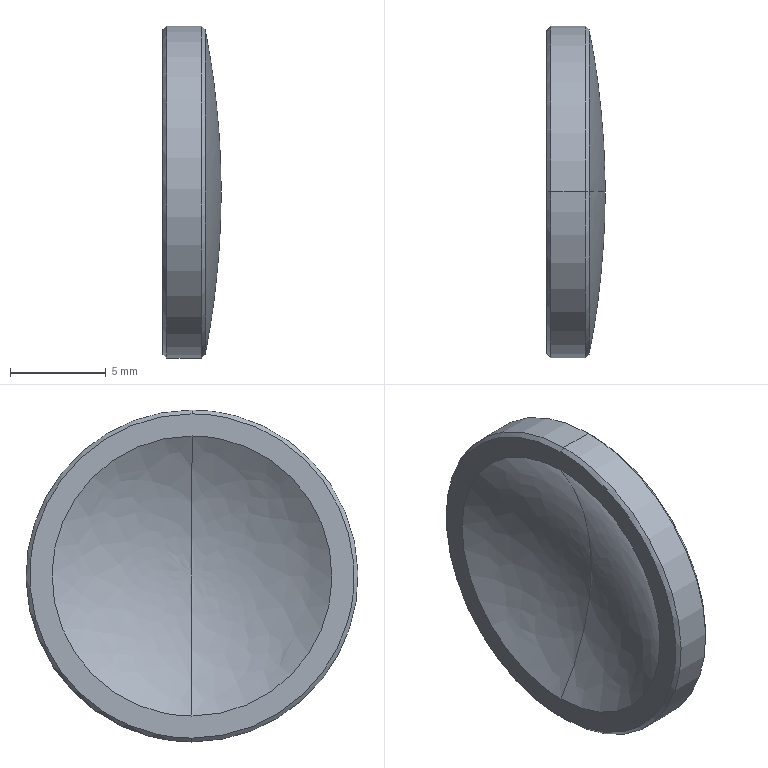Part | SolidWorks | features BaseBody 1 | 1 solid | 11 faces | box 3.031 x 17.3 x 17.3 mm | volume 416.795 mm3 | spline 11
STEP:
#1=CARTESIAN_POINT('',(5.315,0.,-8.45));
#2=VERTEX_POINT('',#1);
#3=CARTESIAN_POINT('',(6.141,0.,0.));
#4=VERTEX_POINT('',#3);
#5=CARTESIAN_POINT('',(-37.512,0.,0.));
#6=DIRECTION('',(0.,-1.,0.));
#7=DIRECTION('',(0.9803,0.,-0.1974));
#8=AXIS2_PLACEMENT_3D('',#5,#6,#7);
#9=CIRCLE('',#8,43.653);
#10=EDGE_CURVE('',#2,#4,#9,.T.);
#11=ORIENTED_EDGE('',*,*,#10,.F.);
#12=CARTESIAN_POINT('',(5.315,0.,8.45));
#13=VERTEX_POINT('',#12);
#14=CARTESIAN_POINT('',(5.315,0.,8.45));
#15=CARTESIAN_POINT('',(5.315,16.9,8.45));
#16=CARTESIAN_POINT('',(5.315,16.9,-8.45));
#17=CARTESIAN_POINT('',(5.315,0.,-8.45));
#18=(BOUNDED_CURVE()B_SPLINE_CURVE(3,(#14,#15,#16,#17),.UNSPECIFIED.,.F.,.F.)B_SPLINE_CURVE_WITH_KNOTS((4,4),(0.,51.9),.UNSPECIFIED.)CURVE()GEOMETRIC_REPRESENTATION_ITEM()RATIONAL_B_SPLINE_CURVE((1.,0.3333,0.3333,1.))REPRESENTATION_ITEM(''));
#19=EDGE_CURVE('',#13,#2,#18,.T.);
#20=ORIENTED_EDGE('',*,*,#19,.F.);
#21=CARTESIAN_POINT('',(-37.512,0.,0.));
#22=DIRECTION('',(0.,1.,0.));
#23=DIRECTION('',(0.9803,0.,0.1974));
#24=AXIS2_PLACEMENT_3D('',#21,#22,#23);
#25=CIRCLE('',#24,43.653);
#26=EDGE_CURVE('',#13,#4,#25,.T.);
#27=ORIENTED_EDGE('',*,*,#26,.T.);
#28=EDGE_LOOP('',(#11,#20,#27));
#29=FACE_OUTER_BOUND('',#28,.T.);
#30=CARTESIAN_POINT('',(5.315,0.,-8.45));
#31=CARTESIAN_POINT('',(5.315,16.9,-8.45));
#32=CARTESIAN_POINT('',(5.315,16.9,8.45));
#33=CARTESIAN_POINT('',(5.315,0.,8.45));
#34=CARTESIAN_POINT('',(5.865,0.,-5.665));
#35=CARTESIAN_POINT('',(5.865,11.329,-5.665));
#36=CARTESIAN_POINT('',(5.865,11.329,5.665));
#37=CARTESIAN_POINT('',(5.865,0.,5.665));
#38=CARTESIAN_POINT('',(6.141,0.,-2.839));
#39=CARTESIAN_POINT('',(6.141,5.678,-2.839));
#40=CARTESIAN_POINT('',(6.141,5.678,2.839));
#41=CARTESIAN_POINT('',(6.141,0.,2.839));
#42=CARTESIAN_POINT('',(6.141,0.,0.));
#43=CARTESIAN_POINT('',(6.141,0.,0.));
#44=CARTESIAN_POINT('',(6.141,0.,0.));
#45=CARTESIAN_POINT('',(6.141,0.,0.));
#46=(BOUNDED_SURFACE()B_SPLINE_SURFACE(3,3,((#30,#31,#32,#33),(#34,#35,#36,#37),(#38,#39,#40,#41),(#42,#43,#44,#45)),.UNSPECIFIED.,.F.,.F.,.T.)B_SPLINE_SURFACE_WITH_KNOTS((4,4),(4,4),(0.,1.),(0.,1.),.UNSPECIFIED.)GEOMETRIC_REPRESENTATION_ITEM()RATIONAL_B_SPLINE_SURFACE(((1.,0.3333,0.3333,1.),(0.9968,0.3323,0.3323,0.9968),(0.9968,0.3323,0.3323,0.9968),(1.,0.3333,0.3333,1.)))REPRESENTATION_ITEM('')SURFACE());
#47=ADVANCED_FACE('',(#29),#46,.F.);
#48=ORIENTED_EDGE('',*,*,#26,.F.);
#49=CARTESIAN_POINT('',(5.315,0.,-8.45));
#50=CARTESIAN_POINT('',(5.315,-16.9,-8.45));
#51=CARTESIAN_POINT('',(5.315,-16.9,8.45));
#52=CARTESIAN_POINT('',(5.315,0.,8.45));
#53=(BOUNDED_CURVE()B_SPLINE_CURVE(3,(#49,#50,#51,#52),.UNSPECIFIED.,.F.,.F.)B_SPLINE_CURVE_WITH_KNOTS((4,4),(0.,51.9),.UNSPECIFIED.)CURVE()GEOMETRIC_REPRESENTATION_ITEM()RATIONAL_B_SPLINE_CURVE((1.,0.3333,0.3333,1.))REPRESENTATION_ITEM(''));
#54=EDGE_CURVE('',#2,#13,#53,.T.);
#55=ORIENTED_EDGE('',*,*,#54,.F.);
#56=ORIENTED_EDGE('',*,*,#10,.T.);
#57=EDGE_LOOP('',(#48,#55,#56));
#58=FACE_OUTER_BOUND('',#57,.T.);
#59=CARTESIAN_POINT('',(5.315,0.,8.45));
#60=CARTESIAN_POINT('',(5.315,-16.9,8.45));
#61=CARTESIAN_POINT('',(5.315,-16.9,-8.45));
#62=CARTESIAN_POINT('',(5.315,0.,-8.45));
#63=CARTESIAN_POINT('',(5.865,0.,5.665));
#64=CARTESIAN_POINT('',(5.865,-11.329,5.665));
#65=CARTESIAN_POINT('',(5.865,-11.329,-5.665));
#66=CARTESIAN_POINT('',(5.865,0.,-5.665));
#67=CARTESIAN_POINT('',(6.141,0.,2.839));
#68=CARTESIAN_POINT('',(6.141,-5.678,2.839));
#69=CARTESIAN_POINT('',(6.141,-5.678,-2.839));
#70=CARTESIAN_POINT('',(6.141,0.,-2.839));
#71=CARTESIAN_POINT('',(6.141,0.,0.));
#72=CARTESIAN_POINT('',(6.141,0.,0.));
#73=CARTESIAN_POINT('',(6.141,0.,0.));
#74=CARTESIAN_POINT('',(6.141,0.,0.));
#75=(BOUNDED_SURFACE()B_SPLINE_SURFACE(3,3,((#59,#60,#61,#62),(#63,#64,#65,#66),(#67,#68,#69,#70),(#71,#72,#73,#74)),.UNSPECIFIED.,.F.,.F.,.F.)B_SPLINE_SURFACE_WITH_KNOTS((4,4),(4,4),(0.,1.),(0.,1.),.UNSPECIFIED.)GEOMETRIC_REPRESENTATION_ITEM()RATIONAL_B_SPLINE_SURFACE(((1.,0.3333,0.3333,1.),(0.9968,0.3323,0.3323,0.9968),(0.9968,0.3323,0.3323,0.9968),(1.,0.3333,0.3333,1.)))REPRESENTATION_ITEM('')SURFACE());
#76=ADVANCED_FACE('',(#58),#75,.F.);
#77=CARTESIAN_POINT('',(5.115,0.,-8.65));
#78=VERTEX_POINT('',#77);
#79=CARTESIAN_POINT('',(5.315,0.,-8.45));
#80=DIRECTION('',(-0.7071,0.,-0.7071));
#81=VECTOR('',#80,1000.);
#82=LINE('',#79,#81);
#83=EDGE_CURVE('',#2,#78,#82,.T.);
#84=ORIENTED_EDGE('',*,*,#83,.F.);
#85=ORIENTED_EDGE('',*,*,#54,.T.);
#86=CARTESIAN_POINT('',(5.115,0.,8.65));
#87=VERTEX_POINT('',#86);
#88=CARTESIAN_POINT('',(5.315,0.,8.45));
#89=DIRECTION('',(-0.7071,0.,0.7071));
#90=VECTOR('',#89,1000.);
#91=LINE('',#88,#90);
#92=EDGE_CURVE('',#13,#87,#91,.T.);
#93=ORIENTED_EDGE('',*,*,#92,.T.);
#94=CARTESIAN_POINT('',(5.115,0.,-8.65));
#95=CARTESIAN_POINT('',(5.115,-17.3,-8.65));
#96=CARTESIAN_POINT('',(5.115,-17.3,8.65));
#97=CARTESIAN_POINT('',(5.115,0.,8.65));
#98=(BOUNDED_CURVE()B_SPLINE_CURVE(3,(#94,#95,#96,#97),.UNSPECIFIED.,.F.,.F.)B_SPLINE_CURVE_WITH_KNOTS((4,4),(0.,51.9),.UNSPECIFIED.)CURVE()GEOMETRIC_REPRESENTATION_ITEM()RATIONAL_B_SPLINE_CURVE((1.,0.3333,0.3333,1.))REPRESENTATION_ITEM(''));
#99=EDGE_CURVE('',#78,#87,#98,.T.);
#100=ORIENTED_EDGE('',*,*,#99,.F.);
#101=EDGE_LOOP('',(#84,#85,#93,#100));
#102=FACE_OUTER_BOUND('',#101,.T.);
#103=CARTESIAN_POINT('',(5.315,0.,-8.45));
#104=CARTESIAN_POINT('',(5.315,-16.9,-8.45));
#105=CARTESIAN_POINT('',(5.315,-16.9,8.45));
#106=CARTESIAN_POINT('',(5.315,0.,8.45));
#107=CARTESIAN_POINT('',(5.115,0.,-8.65));
#108=CARTESIAN_POINT('',(5.115,-17.3,-8.65));
#109=CARTESIAN_POINT('',(5.115,-17.3,8.65));
#110=CARTESIAN_POINT('',(5.115,0.,8.65));
#111=(BOUNDED_SURFACE()B_SPLINE_SURFACE(1,3,((#103,#104,#105,#106),(#107,#108,#109,#110)),.UNSPECIFIED.,.F.,.F.,.F.)B_SPLINE_SURFACE_WITH_KNOTS((2,2),(4,4),(0.,1.),(0.,51.9),.UNSPECIFIED.)GEOMETRIC_REPRESENTATION_ITEM()RATIONAL_B_SPLINE_SURFACE(((1.,0.3333,0.3333,1.),(1.,0.3333,0.3333,1.)))REPRESENTATION_ITEM('')SURFACE());
#112=ADVANCED_FACE('',(#102),#111,.F.);
#113=CARTESIAN_POINT('',(3.31,0.,8.65));
#114=VERTEX_POINT('',#113);
#115=CARTESIAN_POINT('',(3.31,0.,8.65));
#116=DIRECTION('',(1.,0.,0.));
#117=VECTOR('',#116,1000.);
#118=LINE('',#115,#117);
#119=EDGE_CURVE('',#114,#87,#118,.T.);
#120=ORIENTED_EDGE('',*,*,#119,.F.);
#121=CARTESIAN_POINT('',(3.31,0.,-8.65));
#122=VERTEX_POINT('',#121);
#123=CARTESIAN_POINT('',(3.31,0.,-8.65));
#124=CARTESIAN_POINT('',(3.31,-17.3,-8.65));
#125=CARTESIAN_POINT('',(3.31,-17.3,8.65));
#126=CARTESIAN_POINT('',(3.31,0.,8.65));
#127=(BOUNDED_CURVE()B_SPLINE_CURVE(3,(#123,#124,#125,#126),.UNSPECIFIED.,.F.,.F.)B_SPLINE_CURVE_WITH_KNOTS((4,4),(0.,51.9),.UNSPECIFIED.)CURVE()GEOMETRIC_REPRESENTATION_ITEM()RATIONAL_B_SPLINE_CURVE((1.,0.3333,0.3333,1.))REPRESENTATION_ITEM(''));
#128=EDGE_CURVE('',#122,#114,#127,.T.);
#129=ORIENTED_EDGE('',*,*,#128,.F.);
#130=CARTESIAN_POINT('',(3.31,0.,-8.65));
#131=DIRECTION('',(1.,0.,0.));
#132=VECTOR('',#131,1000.);
#133=LINE('',#130,#132);
#134=EDGE_CURVE('',#122,#78,#133,.T.);
#135=ORIENTED_EDGE('',*,*,#134,.T.);
#136=ORIENTED_EDGE('',*,*,#99,.T.);
#137=EDGE_LOOP('',(#120,#129,#135,#136));
#138=FACE_OUTER_BOUND('',#137,.T.);
#139=CARTESIAN_POINT('',(3.31,0.,8.65));
#140=CARTESIAN_POINT('',(3.31,-17.3,8.65));
#141=CARTESIAN_POINT('',(3.31,-17.3,-8.65));
#142=CARTESIAN_POINT('',(3.31,0.,-8.65));
#143=CARTESIAN_POINT('',(5.115,0.,8.65));
#144=CARTESIAN_POINT('',(5.115,-17.3,8.65));
#145=CARTESIAN_POINT('',(5.115,-17.3,-8.65));
#146=CARTESIAN_POINT('',(5.115,0.,-8.65));
#147=(BOUNDED_SURFACE()B_SPLINE_SURFACE(1,3,((#139,#140,#141,#142),(#143,#144,#145,#146)),.UNSPECIFIED.,.F.,.F.,.F.)B_SPLINE_SURFACE_WITH_KNOTS((2,2),(4,4),(0.,1.805),(0.,51.9),.UNSPECIFIED.)GEOMETRIC_REPRESENTATION_ITEM()RATIONAL_B_SPLINE_SURFACE(((1.,0.3333,0.3333,1.),(1.,0.3333,0.3333,1.)))REPRESENTATION_ITEM('')SURFACE());
#148=ADVANCED_FACE('',(#138),#147,.F.);
#149=CARTESIAN_POINT('',(3.31,0.,8.65));
#150=CARTESIAN_POINT('',(3.31,17.3,8.65));
#151=CARTESIAN_POINT('',(3.31,17.3,-8.65));
#152=CARTESIAN_POINT('',(3.31,0.,-8.65));
#153=(BOUNDED_CURVE()B_SPLINE_CURVE(3,(#149,#150,#151,#152),.UNSPECIFIED.,.F.,.T.)B_SPLINE_CURVE_WITH_KNOTS((4,4),(0.,51.9),.UNSPECIFIED.)CURVE()GEOMETRIC_REPRESENTATION_ITEM()RATIONAL_B_SPLINE_CURVE((1.,0.3333,0.3333,1.))REPRESENTATION_ITEM(''));
#154=EDGE_CURVE('',#114,#122,#153,.T.);
#155=ORIENTED_EDGE('',*,*,#154,.F.);
#156=ORIENTED_EDGE('',*,*,#119,.T.);
#157=CARTESIAN_POINT('',(5.115,0.,8.65));
#158=CARTESIAN_POINT('',(5.115,17.3,8.65));
#159=CARTESIAN_POINT('',(5.115,17.3,-8.65));
#160=CARTESIAN_POINT('',(5.115,0.,-8.65));
#161=(BOUNDED_CURVE()B_SPLINE_CURVE(3,(#157,#158,#159,#160),.UNSPECIFIED.,.F.,.T.)B_SPLINE_CURVE_WITH_KNOTS((4,4),(0.,51.9),.UNSPECIFIED.)CURVE()GEOMETRIC_REPRESENTATION_ITEM()RATIONAL_B_SPLINE_CURVE((1.,0.3333,0.3333,1.))REPRESENTATION_ITEM(''));
#162=EDGE_CURVE('',#87,#78,#161,.T.);
#163=ORIENTED_EDGE('',*,*,#162,.T.);
#164=ORIENTED_EDGE('',*,*,#134,.F.);
#165=EDGE_LOOP('',(#155,#156,#163,#164));
#166=FACE_OUTER_BOUND('',#165,.T.);
#167=CARTESIAN_POINT('',(3.31,0.,-8.65));
#168=CARTESIAN_POINT('',(3.31,17.3,-8.65));
#169=CARTESIAN_POINT('',(3.31,17.3,8.65));
#170=CARTESIAN_POINT('',(3.31,0.,8.65));
#171=CARTESIAN_POINT('',(5.115,0.,-8.65));
#172=CARTESIAN_POINT('',(5.115,17.3,-8.65));
#173=CARTESIAN_POINT('',(5.115,17.3,8.65));
#174=CARTESIAN_POINT('',(5.115,0.,8.65));
#175=(BOUNDED_SURFACE()B_SPLINE_SURFACE(1,3,((#167,#168,#169,#170),(#171,#172,#173,#174)),.UNSPECIFIED.,.F.,.F.,.F.)B_SPLINE_SURFACE_WITH_KNOTS((2,2),(4,4),(0.,1.805),(0.,51.9),.UNSPECIFIED.)GEOMETRIC_REPRESENTATION_ITEM()RATIONAL_B_SPLINE_SURFACE(((1.,0.3333,0.3333,1.),(1.,0.3333,0.3333,1.)))REPRESENTATION_ITEM('')SURFACE());
#176=ADVANCED_FACE('',(#166),#175,.F.);
#177=ORIENTED_EDGE('',*,*,#19,.T.);
#178=ORIENTED_EDGE('',*,*,#83,.T.);
#179=ORIENTED_EDGE('',*,*,#162,.F.);
#180=ORIENTED_EDGE('',*,*,#92,.F.);
#181=EDGE_LOOP('',(#177,#178,#179,#180));
#182=FACE_OUTER_BOUND('',#181,.T.);
#183=CARTESIAN_POINT('',(5.315,0.,8.45));
#184=CARTESIAN_POINT('',(5.315,16.9,8.45));
#185=CARTESIAN_POINT('',(5.315,16.9,-8.45));
#186=CARTESIAN_POINT('',(5.315,0.,-8.45));
#187=CARTESIAN_POINT('',(5.115,0.,8.65));
#188=CARTESIAN_POINT('',(5.115,17.3,8.65));
#189=CARTESIAN_POINT('',(5.115,17.3,-8.65));
#190=CARTESIAN_POINT('',(5.115,0.,-8.65));
#191=(BOUNDED_SURFACE()B_SPLINE_SURFACE(1,3,((#183,#184,#185,#186),(#187,#188,#189,#190)),.UNSPECIFIED.,.F.,.F.,.F.)B_SPLINE_SURFACE_WITH_KNOTS((2,2),(4,4),(0.,1.),(0.,51.9),.UNSPECIFIED.)GEOMETRIC_REPRESENTATION_ITEM()RATIONAL_B_SPLINE_SURFACE(((1.,0.3333,0.3333,1.),(1.,0.3333,0.3333,1.)))REPRESENTATION_ITEM('')SURFACE());
#192=ADVANCED_FACE('',(#182),#191,.F.);
#193=CARTESIAN_POINT('',(3.11,0.,8.45));
#194=VERTEX_POINT('',#193);
#195=CARTESIAN_POINT('',(3.11,0.,-8.45));
#196=VERTEX_POINT('',#195);
#197=CARTESIAN_POINT('',(3.11,0.,8.45));
#198=CARTESIAN_POINT('',(3.11,1.106,8.451));
#199=CARTESIAN_POINT('',(3.11,2.212,8.23));
#200=CARTESIAN_POINT('',(3.11,4.256,7.383));
#201=CARTESIAN_POINT('',(3.11,5.193,6.757));
#202=CARTESIAN_POINT('',(3.11,6.757,5.193));
#203=CARTESIAN_POINT('',(3.11,7.383,4.256));
#204=CARTESIAN_POINT('',(3.11,8.23,2.212));
#205=CARTESIAN_POINT('',(3.11,8.45,1.106));
#206=CARTESIAN_POINT('',(3.11,8.45,-1.106));
#207=CARTESIAN_POINT('',(3.11,8.23,-2.212));
#208=CARTESIAN_POINT('',(3.11,7.383,-4.256));
#209=CARTESIAN_POINT('',(3.11,6.757,-5.193));
#210=CARTESIAN_POINT('',(3.11,5.193,-6.757));
#211=CARTESIAN_POINT('',(3.11,4.256,-7.383));
#212=CARTESIAN_POINT('',(3.11,2.212,-8.23));
#213=CARTESIAN_POINT('',(3.11,1.106,-8.451));
#214=CARTESIAN_POINT('',(3.11,0.,-8.45));
#215=B_SPLINE_CURVE_WITH_KNOTS('',3,(#197,#198,#199,#200,#201,#202,#203,#204,#205,#206,#207,#208,#209,#210,#211,#212,#213,#214),.UNSPECIFIED.,.F.,.F.,(4,2,2,2,2,2,2,2,4),(0.,0.125,0.25,0.375,0.5,0.625,0.75,0.875,1.),.UNSPECIFIED.);
#216=EDGE_CURVE('',#194,#196,#215,.T.);
#217=ORIENTED_EDGE('',*,*,#216,.F.);
#218=CARTESIAN_POINT('',(3.11,0.,8.45));
#219=DIRECTION('',(0.7071,0.,0.7071));
#220=VECTOR('',#219,1000.);
#221=LINE('',#218,#220);
#222=EDGE_CURVE('',#194,#114,#221,.T.);
#223=ORIENTED_EDGE('',*,*,#222,.T.);
#224=ORIENTED_EDGE('',*,*,#154,.T.);
#225=CARTESIAN_POINT('',(3.11,0.,-8.45));
#226=DIRECTION('',(0.7071,0.,-0.7071));
#227=VECTOR('',#226,1000.);
#228=LINE('',#225,#227);
#229=EDGE_CURVE('',#196,#122,#228,.T.);
#230=ORIENTED_EDGE('',*,*,#229,.F.);
#231=EDGE_LOOP('',(#217,#223,#224,#230));
#232=FACE_OUTER_BOUND('',#231,.T.);
#233=CARTESIAN_POINT('',(3.11,0.,-8.45));
#234=CARTESIAN_POINT('',(3.11,16.9,-8.45));
#235=CARTESIAN_POINT('',(3.11,16.9,8.45));
#236=CARTESIAN_POINT('',(3.11,0.,8.45));
#237=CARTESIAN_POINT('',(3.31,0.,-8.65));
#238=CARTESIAN_POINT('',(3.31,17.3,-8.65));
#239=CARTESIAN_POINT('',(3.31,17.3,8.65));
#240=CARTESIAN_POINT('',(3.31,0.,8.65));
#241=(BOUNDED_SURFACE()B_SPLINE_SURFACE(1,3,((#233,#234,#235,#236),(#237,#238,#239,#240)),.UNSPECIFIED.,.F.,.F.,.T.)B_SPLINE_SURFACE_WITH_KNOTS((2,2),(4,4),(0.,1.),(0.,51.9),.UNSPECIFIED.)GEOMETRIC_REPRESENTATION_ITEM()RATIONAL_B_SPLINE_SURFACE(((1.,0.3333,0.3333,1.),(1.,0.3333,0.3333,1.)))REPRESENTATION_ITEM('')SURFACE());
#242=ADVANCED_FACE('',(#232),#241,.F.);
#243=ORIENTED_EDGE('',*,*,#222,.F.);
#244=CARTESIAN_POINT('',(3.11,0.,-8.45));
#245=CARTESIAN_POINT('',(3.11,-1.106,-8.451));
#246=CARTESIAN_POINT('',(3.11,-2.212,-8.23));
#247=CARTESIAN_POINT('',(3.11,-4.256,-7.383));
#248=CARTESIAN_POINT('',(3.11,-5.193,-6.757));
#249=CARTESIAN_POINT('',(3.11,-6.757,-5.193));
#250=CARTESIAN_POINT('',(3.11,-7.383,-4.256));
#251=CARTESIAN_POINT('',(3.11,-8.23,-2.212));
#252=CARTESIAN_POINT('',(3.11,-8.45,-1.106));
#253=CARTESIAN_POINT('',(3.11,-8.45,1.106));
#254=CARTESIAN_POINT('',(3.11,-8.23,2.212));
#255=CARTESIAN_POINT('',(3.11,-7.383,4.256));
#256=CARTESIAN_POINT('',(3.11,-6.757,5.193));
#257=CARTESIAN_POINT('',(3.11,-5.193,6.757));
#258=CARTESIAN_POINT('',(3.11,-4.256,7.383));
#259=CARTESIAN_POINT('',(3.11,-2.212,8.23));
#260=CARTESIAN_POINT('',(3.11,-1.106,8.451));
#261=CARTESIAN_POINT('',(3.11,0.,8.45));
#262=B_SPLINE_CURVE_WITH_KNOTS('',3,(#244,#245,#246,#247,#248,#249,#250,#251,#252,#253,#254,#255,#256,#257,#258,#259,#260,#261),.UNSPECIFIED.,.F.,.F.,(4,2,2,2,2,2,2,2,4),(0.,0.125,0.25,0.375,0.5,0.625,0.75,0.875,1.),.UNSPECIFIED.);
#263=EDGE_CURVE('',#196,#194,#262,.T.);
#264=ORIENTED_EDGE('',*,*,#263,.F.);
#265=ORIENTED_EDGE('',*,*,#229,.T.);
#266=ORIENTED_EDGE('',*,*,#128,.T.);
#267=EDGE_LOOP('',(#243,#264,#265,#266));
#268=FACE_OUTER_BOUND('',#267,.T.);
#269=CARTESIAN_POINT('',(3.11,0.,8.45));
#270=CARTESIAN_POINT('',(3.11,-16.9,8.45));
#271=CARTESIAN_POINT('',(3.11,-16.9,-8.45));
#272=CARTESIAN_POINT('',(3.11,0.,-8.45));
#273=CARTESIAN_POINT('',(3.31,0.,8.65));
#274=CARTESIAN_POINT('',(3.31,-17.3,8.65));
#275=CARTESIAN_POINT('',(3.31,-17.3,-8.65));
#276=CARTESIAN_POINT('',(3.31,0.,-8.65));
#277=(BOUNDED_SURFACE()B_SPLINE_SURFACE(1,3,((#269,#270,#271,#272),(#273,#274,#275,#276)),.UNSPECIFIED.,.F.,.F.,.F.)B_SPLINE_SURFACE_WITH_KNOTS((2,2),(4,4),(0.,1.),(0.,51.9),.UNSPECIFIED.)GEOMETRIC_REPRESENTATION_ITEM()RATIONAL_B_SPLINE_SURFACE(((1.,0.3333,0.3333,1.),(1.,0.3333,0.3333,1.)))REPRESENTATION_ITEM('')SURFACE());
#278=ADVANCED_FACE('',(#268),#277,.F.);
#279=CARTESIAN_POINT('',(3.11,0.,7.295));
#280=VERTEX_POINT('',#279);
#281=CARTESIAN_POINT('',(3.11,0.,-7.295));
#282=VERTEX_POINT('',#281);
#283=CARTESIAN_POINT('',(3.11,0.,7.295));
#284=CARTESIAN_POINT('',(3.11,14.591,7.295));
#285=CARTESIAN_POINT('',(3.11,14.591,-7.295));
#286=CARTESIAN_POINT('',(3.11,0.,-7.295));
#287=(BOUNDED_CURVE()B_SPLINE_CURVE(3,(#283,#284,#285,#286),.UNSPECIFIED.,.F.,.F.)B_SPLINE_CURVE_WITH_KNOTS((4,4),(0.,1.),.UNSPECIFIED.)CURVE()GEOMETRIC_REPRESENTATION_ITEM()RATIONAL_B_SPLINE_CURVE((1.,0.3333,0.3333,1.))REPRESENTATION_ITEM(''));
#288=EDGE_CURVE('',#280,#282,#287,.T.);
#289=ORIENTED_EDGE('',*,*,#288,.F.);
#290=CARTESIAN_POINT('',(3.11,0.,-7.295));
#291=CARTESIAN_POINT('',(3.11,-14.591,-7.295));
#292=CARTESIAN_POINT('',(3.11,-14.591,7.295));
#293=CARTESIAN_POINT('',(3.11,0.,7.295));
#294=(BOUNDED_CURVE()B_SPLINE_CURVE(3,(#290,#291,#292,#293),.UNSPECIFIED.,.F.,.F.)B_SPLINE_CURVE_WITH_KNOTS((4,4),(0.,1.),.UNSPECIFIED.)CURVE()GEOMETRIC_REPRESENTATION_ITEM()RATIONAL_B_SPLINE_CURVE((1.,0.3333,0.3333,1.))REPRESENTATION_ITEM(''));
#295=EDGE_CURVE('',#282,#280,#294,.T.);
#296=ORIENTED_EDGE('',*,*,#295,.F.);
#297=EDGE_LOOP('',(#289,#296));
#298=FACE_BOUND('',#297,.T.);
#299=ORIENTED_EDGE('',*,*,#263,.T.);
#300=ORIENTED_EDGE('',*,*,#216,.T.);
#301=EDGE_LOOP('',(#299,#300));
#302=FACE_OUTER_BOUND('',#301,.T.);
#303=CARTESIAN_POINT('',(3.11,-8.534,8.535));
#304=CARTESIAN_POINT('',(3.11,8.534,8.535));
#305=CARTESIAN_POINT('',(3.11,-8.534,-8.535));
#306=CARTESIAN_POINT('',(3.11,8.534,-8.535));
#307=B_SPLINE_SURFACE_WITH_KNOTS('',1,1,((#303,#304),(#305,#306)),.UNSPECIFIED.,.F.,.F.,.F.,(2,2),(2,2),(-8.535,8.535),(-8.534,8.534),.UNSPECIFIED.);
#308=ADVANCED_FACE('',(#298,#302),#307,.F.);
#309=CARTESIAN_POINT('',(5.341,0.,0.));
#310=VERTEX_POINT('',#309);
#311=CARTESIAN_POINT('',(-7.703,0.,0.));
#312=DIRECTION('',(0.,-1.,0.));
#313=DIRECTION('',(0.8223,0.,-0.5691));
#314=AXIS2_PLACEMENT_3D('',#311,#312,#313);
#315=CIRCLE('',#314,13.044);
#316=EDGE_CURVE('',#282,#310,#315,.T.);
#317=ORIENTED_EDGE('',*,*,#316,.F.);
#318=ORIENTED_EDGE('',*,*,#295,.T.);
#319=CARTESIAN_POINT('',(-7.703,0.,0.));
#320=DIRECTION('',(0.,1.,0.));
#321=DIRECTION('',(0.8223,0.,0.5691));
#322=AXIS2_PLACEMENT_3D('',#319,#320,#321);
#323=CIRCLE('',#322,13.044);
#324=EDGE_CURVE('',#280,#310,#323,.T.);
#325=ORIENTED_EDGE('',*,*,#324,.T.);
#326=EDGE_LOOP('',(#317,#318,#325));
#327=FACE_OUTER_BOUND('',#326,.T.);
#328=CARTESIAN_POINT('',(3.11,0.,7.295));
#329=CARTESIAN_POINT('',(3.11,-14.591,7.295));
#330=CARTESIAN_POINT('',(3.11,-14.591,-7.295));
#331=CARTESIAN_POINT('',(3.11,0.,-7.295));
#332=CARTESIAN_POINT('',(4.575,0.,5.124));
#333=CARTESIAN_POINT('',(4.575,-10.248,5.124));
#334=CARTESIAN_POINT('',(4.575,-10.248,-5.124));
#335=CARTESIAN_POINT('',(4.575,0.,-5.124));
#336=CARTESIAN_POINT('',(5.341,0.,2.619));
#337=CARTESIAN_POINT('',(5.341,-5.239,2.619));
#338=CARTESIAN_POINT('',(5.341,-5.239,-2.619));
#339=CARTESIAN_POINT('',(5.341,0.,-2.619));
#340=CARTESIAN_POINT('',(5.341,0.,0.));
#341=CARTESIAN_POINT('',(5.341,0.,0.));
#342=CARTESIAN_POINT('',(5.341,0.,0.));
#343=CARTESIAN_POINT('',(5.341,0.,0.));
#344=(BOUNDED_SURFACE()B_SPLINE_SURFACE(3,3,((#328,#329,#330,#331),(#332,#333,#334,#335),(#336,#337,#338,#339),(#340,#341,#342,#343)),.UNSPECIFIED.,.F.,.F.,.T.)B_SPLINE_SURFACE_WITH_KNOTS((4,4),(4,4),(0.,1.),(0.,1.),.UNSPECIFIED.)GEOMETRIC_REPRESENTATION_ITEM()RATIONAL_B_SPLINE_SURFACE(((1.,0.3333,0.3333,1.),(0.9709,0.3236,0.3236,0.9709),(0.9709,0.3236,0.3236,0.9709),(1.,0.3333,0.3333,1.)))REPRESENTATION_ITEM('')SURFACE());
#345=ADVANCED_FACE('',(#327),#344,.T.);
#346=ORIENTED_EDGE('',*,*,#324,.F.);
#347=ORIENTED_EDGE('',*,*,#288,.T.);
#348=ORIENTED_EDGE('',*,*,#316,.T.);
#349=EDGE_LOOP('',(#346,#347,#348));
#350=FACE_OUTER_BOUND('',#349,.T.);
#351=CARTESIAN_POINT('',(3.11,0.,-7.295));
#352=CARTESIAN_POINT('',(3.11,14.591,-7.295));
#353=CARTESIAN_POINT('',(3.11,14.591,7.295));
#354=CARTESIAN_POINT('',(3.11,0.,7.295));
#355=CARTESIAN_POINT('',(4.575,0.,-5.124));
#356=CARTESIAN_POINT('',(4.575,10.248,-5.124));
#357=CARTESIAN_POINT('',(4.575,10.248,5.124));
#358=CARTESIAN_POINT('',(4.575,0.,5.124));
#359=CARTESIAN_POINT('',(5.341,0.,-2.619));
#360=CARTESIAN_POINT('',(5.341,5.239,-2.619));
#361=CARTESIAN_POINT('',(5.341,5.239,2.619));
#362=CARTESIAN_POINT('',(5.341,0.,2.619));
#363=CARTESIAN_POINT('',(5.341,0.,0.));
#364=CARTESIAN_POINT('',(5.341,0.,0.));
#365=CARTESIAN_POINT('',(5.341,0.,0.));
#366=CARTESIAN_POINT('',(5.341,0.,0.));
#367=(BOUNDED_SURFACE()B_SPLINE_SURFACE(3,3,((#351,#352,#353,#354),(#355,#356,#357,#358),(#359,#360,#361,#362),(#363,#364,#365,#366)),.UNSPECIFIED.,.F.,.F.,.F.)B_SPLINE_SURFACE_WITH_KNOTS((4,4),(4,4),(0.,1.),(0.,1.),.UNSPECIFIED.)GEOMETRIC_REPRESENTATION_ITEM()RATIONAL_B_SPLINE_SURFACE(((1.,0.3333,0.3333,1.),(0.9709,0.3236,0.3236,0.9709),(0.9709,0.3236,0.3236,0.9709),(1.,0.3333,0.3333,1.)))REPRESENTATION_ITEM('')SURFACE());
#368=ADVANCED_FACE('',(#350),#367,.T.);
#369=CLOSED_SHELL('',(#47,#76,#112,#148,#176,#192,#242,#278,#308,#345,#368));
#370=MANIFOLD_SOLID_BREP('',#369);
#371=CARTESIAN_POINT('',(0.,0.,0.));
#372=DIRECTION('',(0.,0.,1.));
#373=DIRECTION('',(1.,0.,0.));
#374=AXIS2_PLACEMENT_3D('',#371,#372,#373);
#375=(LENGTH_UNIT()NAMED_UNIT(*)SI_UNIT(.MILLI.,.METRE.));
#376=UNCERTAINTY_MEASURE_WITH_UNIT(LENGTH_MEASURE(0.00001),#375,'','');
#377=(NAMED_UNIT(*)PLANE_ANGLE_UNIT()SI_UNIT($,.RADIAN.));
#378=(NAMED_UNIT(*)SI_UNIT($,.STERADIAN.)SOLID_ANGLE_UNIT());
#379=(GEOMETRIC_REPRESENTATION_CONTEXT(3)GLOBAL_UNCERTAINTY_ASSIGNED_CONTEXT((#376))GLOBAL_UNIT_ASSIGNED_CONTEXT((#375,#377,#378))REPRESENTATION_CONTEXT('',''));
#380=ADVANCED_BREP_SHAPE_REPRESENTATION('',(#370,#374),#379);